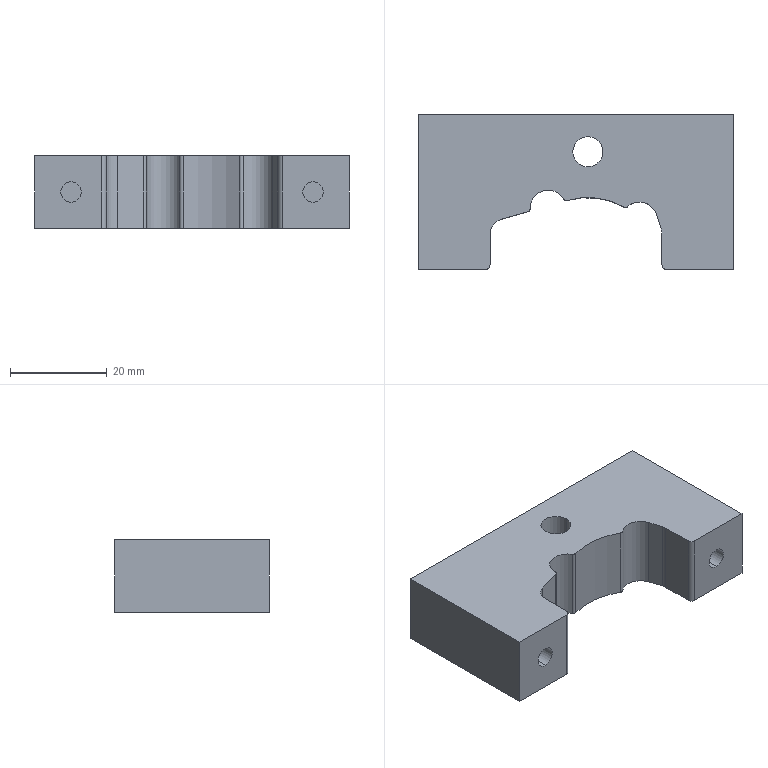NC program | Mastercam | posted with a generic post
Lines 1 to 24 of 2481:
%
O0000()
(MATERIAL - ALUMINUM MM - 2024)
( T1 | 50 FM | H1 )
( T9 | 8 FEMR | H9 | XY STOCK TO LEAVE - .1 | Z STOCK TO LEAVE - 0. )
( T3 | 5 FEMF | H3 | XY STOCK TO LEAVE - .1 | Z STOCK TO LEAVE - 0. )
( T5 | 8 CHM | H5 )
( T11 | 6.2 DR | H11 )
( T10 | 8 FEMF | H10 | D10 | WEAR COMP | TOOL DIA. - 8. )
( T15 | 4.2 DR | H15 )
( T16 | M5 X 0.8 RH | H16 )
N100 G21
N110 G0 G17 G40 G49 G80 G90
N120 T1 M6
N130 G0 G90 G54 X75. Y0. A0. S5000 M3
N140 G43 H1 Z50.
N150 Z2.
N160 G1 Z0. F2000.
N170 X-75. F700.
N180 G0 Z50.
N190 M5
N200 G91 G28 Z0.
N210 A0.
N220 M01